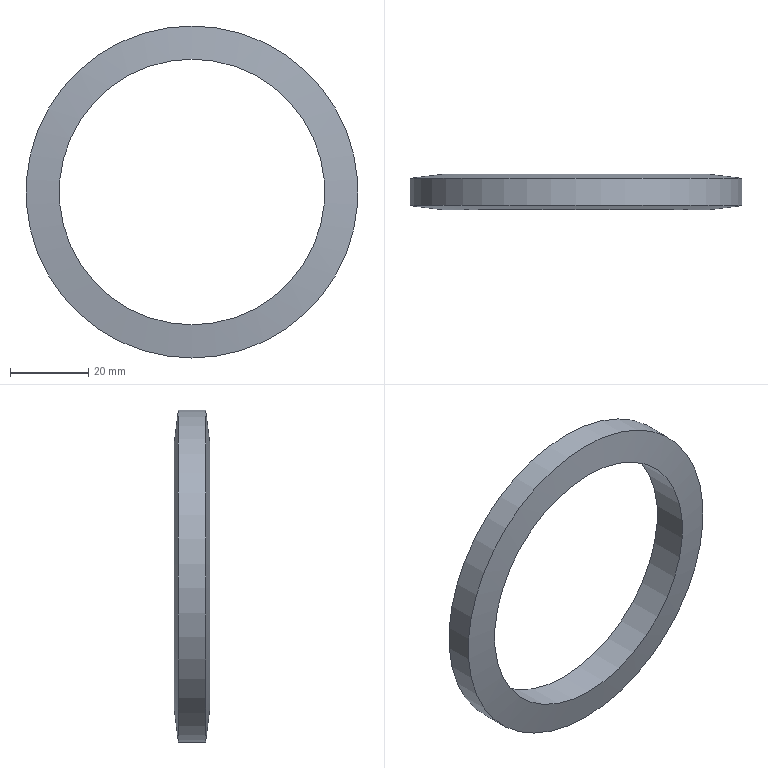Part | NX | 1 solid | 4 faces | box 85 x 9.087 x 85 mm | volume 16353 mm3 | cone 2 | cylinder 2 | commonest cylinder face diameters 68 x1 85 x1
STEP:
#1=CARTESIAN_POINT('',(0.,277.1,42.5));
#2=VERTEX_POINT('',#1);
#3=CARTESIAN_POINT('',(0.,277.1,0.));
#4=DIRECTION('',(0.,1.,0.));
#5=DIRECTION('',(0.,0.,1.));
#6=AXIS2_PLACEMENT_3D('',#3,#4,#5);
#7=CIRCLE('',#6,42.5);
#8=EDGE_CURVE('',#2,#2,#7,.T.);
#9=ORIENTED_EDGE('',*,*,#8,.T.);
#10=EDGE_LOOP('',(#9));
#11=FACE_BOUND('',#10,.T.);
#12=CARTESIAN_POINT('',(0.,278.144,34.));
#13=VERTEX_POINT('',#12);
#14=CARTESIAN_POINT('',(0.,278.144,0.));
#15=DIRECTION('',(0.,1.,0.));
#16=DIRECTION('',(0.,0.,1.));
#17=AXIS2_PLACEMENT_3D('',#14,#15,#16);
#18=CIRCLE('',#17,34.);
#19=EDGE_CURVE('',#13,#13,#18,.T.);
#20=ORIENTED_EDGE('',*,*,#19,.F.);
#21=EDGE_LOOP('',(#20));
#22=FACE_BOUND('',#21,.T.);
#23=CARTESIAN_POINT('',(0.,278.144,0.));
#24=DIRECTION('',(0.,-1.,0.));
#25=DIRECTION('',(0.,0.,1.));
#26=AXIS2_PLACEMENT_3D('',#23,#24,#25);
#27=CONICAL_SURFACE('',#26,34.,83.);
#28=ADVANCED_FACE('',(#11,#22),#27,.T.);
#29=CARTESIAN_POINT('',(0.,270.1,42.5));
#30=VERTEX_POINT('',#29);
#31=CARTESIAN_POINT('',(0.,270.1,0.));
#32=DIRECTION('',(0.,1.,0.));
#33=DIRECTION('',(0.,0.,1.));
#34=AXIS2_PLACEMENT_3D('',#31,#32,#33);
#35=CIRCLE('',#34,42.5);
#36=EDGE_CURVE('',#30,#30,#35,.T.);
#37=ORIENTED_EDGE('',*,*,#36,.T.);
#38=EDGE_LOOP('',(#37));
#39=FACE_BOUND('',#38,.T.);
#40=ORIENTED_EDGE('',*,*,#8,.F.);
#41=EDGE_LOOP('',(#40));
#42=FACE_BOUND('',#41,.T.);
#43=CARTESIAN_POINT('',(0.,221.87,0.));
#44=DIRECTION('',(0.,1.,0.));
#45=DIRECTION('',(0.,0.,-1.));
#46=AXIS2_PLACEMENT_3D('',#43,#44,#45);
#47=CYLINDRICAL_SURFACE('',#46,42.5);
#48=ADVANCED_FACE('',(#39,#42),#47,.T.);
#49=CARTESIAN_POINT('',(0.,269.056,34.));
#50=VERTEX_POINT('',#49);
#51=CARTESIAN_POINT('',(0.,269.056,0.));
#52=DIRECTION('',(0.,1.,0.));
#53=DIRECTION('',(0.,0.,1.));
#54=AXIS2_PLACEMENT_3D('',#51,#52,#53);
#55=CIRCLE('',#54,34.);
#56=EDGE_CURVE('',#50,#50,#55,.T.);
#57=ORIENTED_EDGE('',*,*,#56,.T.);
#58=EDGE_LOOP('',(#57));
#59=FACE_BOUND('',#58,.T.);
#60=ORIENTED_EDGE('',*,*,#36,.F.);
#61=EDGE_LOOP('',(#60));
#62=FACE_BOUND('',#61,.T.);
#63=CARTESIAN_POINT('',(0.,270.1,0.));
#64=DIRECTION('',(0.,1.,0.));
#65=DIRECTION('',(0.,0.,-1.));
#66=AXIS2_PLACEMENT_3D('',#63,#64,#65);
#67=CONICAL_SURFACE('',#66,42.5,83.);
#68=ADVANCED_FACE('',(#59,#62),#67,.T.);
#69=ORIENTED_EDGE('',*,*,#19,.T.);
#70=EDGE_LOOP('',(#69));
#71=FACE_BOUND('',#70,.T.);
#72=ORIENTED_EDGE('',*,*,#56,.F.);
#73=EDGE_LOOP('',(#72));
#74=FACE_BOUND('',#73,.T.);
#75=CARTESIAN_POINT('',(0.,221.87,0.));
#76=DIRECTION('',(0.,1.,0.));
#77=DIRECTION('',(0.,0.,-1.));
#78=AXIS2_PLACEMENT_3D('',#75,#76,#77);
#79=CYLINDRICAL_SURFACE('',#78,34.);
#80=ADVANCED_FACE('',(#71,#74),#79,.F.);
#81=CLOSED_SHELL('',(#28,#48,#68,#80));
#82=MANIFOLD_SOLID_BREP('',#81);
#83=(LENGTH_UNIT()NAMED_UNIT(*)SI_UNIT(.MILLI.,.METRE.));
#84=UNCERTAINTY_MEASURE_WITH_UNIT(LENGTH_MEASURE(0.00002),#83,'','');
#85=(NAMED_UNIT(*)PLANE_ANGLE_UNIT()SI_UNIT($,.RADIAN.));
#86=PLANE_ANGLE_MEASURE_WITH_UNIT(PLANE_ANGLE_MEASURE(0.01745),#85);
#87=DIMENSIONAL_EXPONENTS(0.,0.,0.,0.,0.,0.,0.);
#88=(CONVERSION_BASED_UNIT('DEGREE',#86)NAMED_UNIT(#87)PLANE_ANGLE_UNIT());
#89=(NAMED_UNIT(*)SI_UNIT($,.STERADIAN.)SOLID_ANGLE_UNIT());
#90=(GEOMETRIC_REPRESENTATION_CONTEXT(3)GLOBAL_UNCERTAINTY_ASSIGNED_CONTEXT((#84))GLOBAL_UNIT_ASSIGNED_CONTEXT((#83,#88,#89))REPRESENTATION_CONTEXT('',''));
#91=ADVANCED_BREP_SHAPE_REPRESENTATION('',(#82),#90);